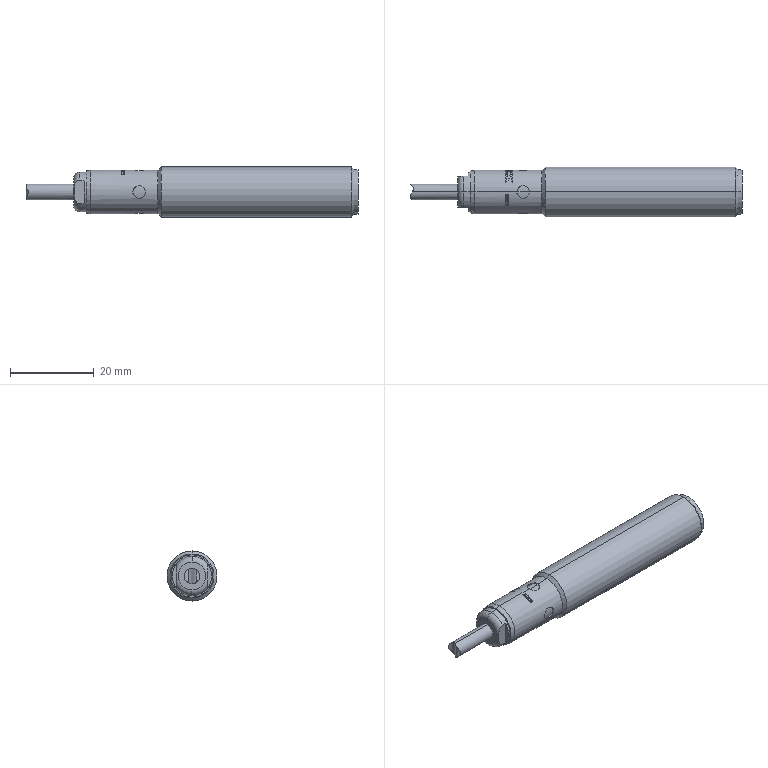Part | SolidWorks | features BaseBody 1 | 1 solid | 140 faces | box 79.369 x 12 x 12 mm | volume 7140 mm3 | plane 74 | cylinder 31 | spline 25 | cone 8 | torus 2 | commonest cylinder face diameters 10.48 x9 3 x8 10 x5 3.7 x2 9.4 x2 10.5 x2